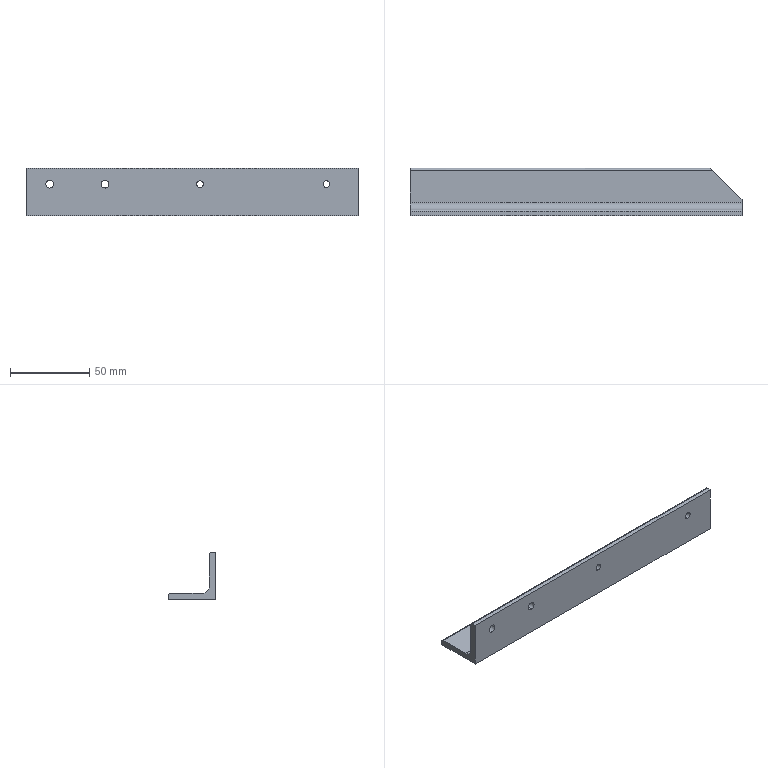Part | NX | features BREP 1 | 1 solid | 20 faces | box 210 x 30 x 30 mm | volume 46732 mm3 | cylinder 11 | plane 9 | commonest cylinder face diameters 4.2 x4 5 x4 2.667 x2 9 x1
STEP:
#1=CARTESIAN_POINT('',(15.,4.,22.5));
#2=VERTEX_POINT('',#1);
#3=CARTESIAN_POINT('',(15.,4.,17.5));
#4=VERTEX_POINT('',#3);
#5=CARTESIAN_POINT('',(15.,4.,20.));
#6=DIRECTION('',(0.,-1.,0.));
#7=DIRECTION('',(0.,0.,-1.));
#8=AXIS2_PLACEMENT_3D('',#5,#6,#7);
#9=CIRCLE('',#8,2.5);
#10=EDGE_CURVE('',#2,#4,#9,.T.);
#11=ORIENTED_EDGE('',*,*,#10,.F.);
#12=CARTESIAN_POINT('',(15.,0.,22.5));
#13=VERTEX_POINT('',#12);
#14=CARTESIAN_POINT('',(15.,0.,22.5));
#15=DIRECTION('',(0.,-1.,0.));
#16=VECTOR('',#15,1000.);
#17=LINE('',#14,#16);
#18=EDGE_CURVE('',#2,#13,#17,.T.);
#19=ORIENTED_EDGE('',*,*,#18,.T.);
#20=CARTESIAN_POINT('',(15.,0.,17.5));
#21=VERTEX_POINT('',#20);
#22=CARTESIAN_POINT('',(15.,0.,20.));
#23=DIRECTION('',(0.,-1.,0.));
#24=DIRECTION('',(0.,0.,-1.));
#25=AXIS2_PLACEMENT_3D('',#22,#23,#24);
#26=CIRCLE('',#25,2.5);
#27=EDGE_CURVE('',#13,#21,#26,.T.);
#28=ORIENTED_EDGE('',*,*,#27,.T.);
#29=CARTESIAN_POINT('',(15.,0.,17.5));
#30=DIRECTION('',(0.,-1.,0.));
#31=VECTOR('',#30,1000.);
#32=LINE('',#29,#31);
#33=EDGE_CURVE('',#4,#21,#32,.T.);
#34=ORIENTED_EDGE('',*,*,#33,.F.);
#35=EDGE_LOOP('',(#11,#19,#28,#34));
#36=FACE_BOUND('',#35,.T.);
#37=CARTESIAN_POINT('',(15.,0.,20.));
#38=DIRECTION('',(0.,-1.,0.));
#39=DIRECTION('',(0.,0.,-1.));
#40=AXIS2_PLACEMENT_3D('',#37,#38,#39);
#41=CYLINDRICAL_SURFACE('',#40,2.5);
#42=ADVANCED_FACE('',(#36),#41,.F.);
#43=CARTESIAN_POINT('',(50.,4.,22.5));
#44=VERTEX_POINT('',#43);
#45=CARTESIAN_POINT('',(50.,4.,17.5));
#46=VERTEX_POINT('',#45);
#47=CARTESIAN_POINT('',(50.,4.,20.));
#48=DIRECTION('',(0.,-1.,0.));
#49=DIRECTION('',(0.,0.,-1.));
#50=AXIS2_PLACEMENT_3D('',#47,#48,#49);
#51=CIRCLE('',#50,2.5);
#52=EDGE_CURVE('',#44,#46,#51,.T.);
#53=ORIENTED_EDGE('',*,*,#52,.F.);
#54=CARTESIAN_POINT('',(50.,0.,22.5));
#55=VERTEX_POINT('',#54);
#56=CARTESIAN_POINT('',(50.,0.,22.5));
#57=DIRECTION('',(0.,-1.,0.));
#58=VECTOR('',#57,1000.);
#59=LINE('',#56,#58);
#60=EDGE_CURVE('',#44,#55,#59,.T.);
#61=ORIENTED_EDGE('',*,*,#60,.T.);
#62=CARTESIAN_POINT('',(50.,0.,17.5));
#63=VERTEX_POINT('',#62);
#64=CARTESIAN_POINT('',(50.,0.,20.));
#65=DIRECTION('',(0.,-1.,0.));
#66=DIRECTION('',(0.,0.,-1.));
#67=AXIS2_PLACEMENT_3D('',#64,#65,#66);
#68=CIRCLE('',#67,2.5);
#69=EDGE_CURVE('',#55,#63,#68,.T.);
#70=ORIENTED_EDGE('',*,*,#69,.T.);
#71=CARTESIAN_POINT('',(50.,0.,17.5));
#72=DIRECTION('',(0.,-1.,0.));
#73=VECTOR('',#72,1000.);
#74=LINE('',#71,#73);
#75=EDGE_CURVE('',#46,#63,#74,.T.);
#76=ORIENTED_EDGE('',*,*,#75,.F.);
#77=EDGE_LOOP('',(#53,#61,#70,#76));
#78=FACE_BOUND('',#77,.T.);
#79=CARTESIAN_POINT('',(50.,0.,20.));
#80=DIRECTION('',(0.,-1.,0.));
#81=DIRECTION('',(0.,0.,-1.));
#82=AXIS2_PLACEMENT_3D('',#79,#80,#81);
#83=CYLINDRICAL_SURFACE('',#82,2.5);
#84=ADVANCED_FACE('',(#78),#83,.F.);
#85=CARTESIAN_POINT('',(190.,4.,22.1));
#86=VERTEX_POINT('',#85);
#87=CARTESIAN_POINT('',(190.,4.,17.9));
#88=VERTEX_POINT('',#87);
#89=CARTESIAN_POINT('',(190.,4.,20.));
#90=DIRECTION('',(0.,-1.,0.));
#91=DIRECTION('',(0.,0.,-1.));
#92=AXIS2_PLACEMENT_3D('',#89,#90,#91);
#93=CIRCLE('',#92,2.1);
#94=EDGE_CURVE('',#86,#88,#93,.T.);
#95=ORIENTED_EDGE('',*,*,#94,.F.);
#96=CARTESIAN_POINT('',(190.,0.,22.1));
#97=VERTEX_POINT('',#96);
#98=CARTESIAN_POINT('',(190.,0.,22.1));
#99=DIRECTION('',(0.,-1.,0.));
#100=VECTOR('',#99,1000.);
#101=LINE('',#98,#100);
#102=EDGE_CURVE('',#86,#97,#101,.T.);
#103=ORIENTED_EDGE('',*,*,#102,.T.);
#104=CARTESIAN_POINT('',(190.,0.,17.9));
#105=VERTEX_POINT('',#104);
#106=CARTESIAN_POINT('',(190.,0.,20.));
#107=DIRECTION('',(0.,-1.,0.));
#108=DIRECTION('',(0.,0.,-1.));
#109=AXIS2_PLACEMENT_3D('',#106,#107,#108);
#110=CIRCLE('',#109,2.1);
#111=EDGE_CURVE('',#97,#105,#110,.T.);
#112=ORIENTED_EDGE('',*,*,#111,.T.);
#113=CARTESIAN_POINT('',(190.,0.,17.9));
#114=DIRECTION('',(0.,-1.,0.));
#115=VECTOR('',#114,1000.);
#116=LINE('',#113,#115);
#117=EDGE_CURVE('',#88,#105,#116,.T.);
#118=ORIENTED_EDGE('',*,*,#117,.F.);
#119=EDGE_LOOP('',(#95,#103,#112,#118));
#120=FACE_BOUND('',#119,.T.);
#121=CARTESIAN_POINT('',(190.,0.,20.));
#122=DIRECTION('',(0.,-1.,0.));
#123=DIRECTION('',(0.,0.,-1.));
#124=AXIS2_PLACEMENT_3D('',#121,#122,#123);
#125=CYLINDRICAL_SURFACE('',#124,2.1);
#126=ADVANCED_FACE('',(#120),#125,.F.);
#127=CARTESIAN_POINT('',(110.,4.,22.1));
#128=VERTEX_POINT('',#127);
#129=CARTESIAN_POINT('',(110.,4.,17.9));
#130=VERTEX_POINT('',#129);
#131=CARTESIAN_POINT('',(110.,4.,20.));
#132=DIRECTION('',(0.,-1.,0.));
#133=DIRECTION('',(0.,0.,-1.));
#134=AXIS2_PLACEMENT_3D('',#131,#132,#133);
#135=CIRCLE('',#134,2.1);
#136=EDGE_CURVE('',#128,#130,#135,.T.);
#137=ORIENTED_EDGE('',*,*,#136,.F.);
#138=CARTESIAN_POINT('',(110.,0.,22.1));
#139=VERTEX_POINT('',#138);
#140=CARTESIAN_POINT('',(110.,0.,22.1));
#141=DIRECTION('',(0.,-1.,0.));
#142=VECTOR('',#141,1000.);
#143=LINE('',#140,#142);
#144=EDGE_CURVE('',#128,#139,#143,.T.);
#145=ORIENTED_EDGE('',*,*,#144,.T.);
#146=CARTESIAN_POINT('',(110.,0.,17.9));
#147=VERTEX_POINT('',#146);
#148=CARTESIAN_POINT('',(110.,0.,20.));
#149=DIRECTION('',(0.,-1.,0.));
#150=DIRECTION('',(0.,0.,-1.));
#151=AXIS2_PLACEMENT_3D('',#148,#149,#150);
#152=CIRCLE('',#151,2.1);
#153=EDGE_CURVE('',#139,#147,#152,.T.);
#154=ORIENTED_EDGE('',*,*,#153,.T.);
#155=CARTESIAN_POINT('',(110.,0.,17.9));
#156=DIRECTION('',(0.,-1.,0.));
#157=VECTOR('',#156,1000.);
#158=LINE('',#155,#157);
#159=EDGE_CURVE('',#130,#147,#158,.T.);
#160=ORIENTED_EDGE('',*,*,#159,.F.);
#161=EDGE_LOOP('',(#137,#145,#154,#160));
#162=FACE_BOUND('',#161,.T.);
#163=CARTESIAN_POINT('',(110.,0.,20.));
#164=DIRECTION('',(0.,-1.,0.));
#165=DIRECTION('',(0.,0.,-1.));
#166=AXIS2_PLACEMENT_3D('',#163,#164,#165);
#167=CYLINDRICAL_SURFACE('',#166,2.1);
#168=ADVANCED_FACE('',(#162),#167,.F.);
#169=CARTESIAN_POINT('',(0.,0.,30.));
#170=VERTEX_POINT('',#169);
#171=CARTESIAN_POINT('',(0.,0.,0.));
#172=VERTEX_POINT('',#171);
#173=CARTESIAN_POINT('',(0.,0.,0.));
#174=DIRECTION('',(0.,0.,-1.));
#175=VECTOR('',#174,1000.);
#176=LINE('',#173,#175);
#177=EDGE_CURVE('',#170,#172,#176,.T.);
#178=ORIENTED_EDGE('',*,*,#177,.T.);
#179=CARTESIAN_POINT('',(210.,0.,0.));
#180=VERTEX_POINT('',#179);
#181=CARTESIAN_POINT('',(210.,0.,0.));
#182=DIRECTION('',(-1.,0.,0.));
#183=VECTOR('',#182,1000.);
#184=LINE('',#181,#183);
#185=EDGE_CURVE('',#180,#172,#184,.T.);
#186=ORIENTED_EDGE('',*,*,#185,.F.);
#187=CARTESIAN_POINT('',(210.,0.,30.));
#188=VERTEX_POINT('',#187);
#189=CARTESIAN_POINT('',(210.,0.,0.));
#190=DIRECTION('',(0.,0.,-1.));
#191=VECTOR('',#190,1000.);
#192=LINE('',#189,#191);
#193=EDGE_CURVE('',#188,#180,#192,.T.);
#194=ORIENTED_EDGE('',*,*,#193,.F.);
#195=CARTESIAN_POINT('',(210.,0.,30.));
#196=DIRECTION('',(-1.,0.,0.));
#197=VECTOR('',#196,1000.);
#198=LINE('',#195,#197);
#199=EDGE_CURVE('',#188,#170,#198,.T.);
#200=ORIENTED_EDGE('',*,*,#199,.T.);
#201=EDGE_LOOP('',(#178,#186,#194,#200));
#202=FACE_BOUND('',#201,.T.);
#203=CARTESIAN_POINT('',(15.,0.,20.));
#204=DIRECTION('',(0.,-1.,0.));
#205=DIRECTION('',(0.,0.,-1.));
#206=AXIS2_PLACEMENT_3D('',#203,#204,#205);
#207=CIRCLE('',#206,2.5);
#208=EDGE_CURVE('',#21,#13,#207,.T.);
#209=ORIENTED_EDGE('',*,*,#208,.F.);
#210=ORIENTED_EDGE('',*,*,#27,.F.);
#211=EDGE_LOOP('',(#209,#210));
#212=FACE_BOUND('',#211,.T.);
#213=CARTESIAN_POINT('',(50.,0.,20.));
#214=DIRECTION('',(0.,-1.,0.));
#215=DIRECTION('',(0.,0.,-1.));
#216=AXIS2_PLACEMENT_3D('',#213,#214,#215);
#217=CIRCLE('',#216,2.5);
#218=EDGE_CURVE('',#63,#55,#217,.T.);
#219=ORIENTED_EDGE('',*,*,#218,.F.);
#220=ORIENTED_EDGE('',*,*,#69,.F.);
#221=EDGE_LOOP('',(#219,#220));
#222=FACE_BOUND('',#221,.T.);
#223=CARTESIAN_POINT('',(190.,0.,20.));
#224=DIRECTION('',(0.,-1.,0.));
#225=DIRECTION('',(0.,0.,-1.));
#226=AXIS2_PLACEMENT_3D('',#223,#224,#225);
#227=CIRCLE('',#226,2.1);
#228=EDGE_CURVE('',#105,#97,#227,.T.);
#229=ORIENTED_EDGE('',*,*,#228,.F.);
#230=ORIENTED_EDGE('',*,*,#111,.F.);
#231=EDGE_LOOP('',(#229,#230));
#232=FACE_BOUND('',#231,.T.);
#233=CARTESIAN_POINT('',(110.,0.,20.));
#234=DIRECTION('',(0.,-1.,0.));
#235=DIRECTION('',(0.,0.,-1.));
#236=AXIS2_PLACEMENT_3D('',#233,#234,#235);
#237=CIRCLE('',#236,2.1);
#238=EDGE_CURVE('',#147,#139,#237,.T.);
#239=ORIENTED_EDGE('',*,*,#238,.F.);
#240=ORIENTED_EDGE('',*,*,#153,.F.);
#241=EDGE_LOOP('',(#239,#240));
#242=FACE_BOUND('',#241,.T.);
#243=CARTESIAN_POINT('',(210.,0.,0.));
#244=DIRECTION('',(0.,1.,0.));
#245=DIRECTION('',(1.,0.,0.));
#246=AXIS2_PLACEMENT_3D('',#243,#244,#245);
#247=PLANE('',#246);
#248=ADVANCED_FACE('',(#202,#212,#222,#232,#242),#247,.F.);
#249=CARTESIAN_POINT('',(190.,30.,0.));
#250=VERTEX_POINT('',#249);
#251=CARTESIAN_POINT('',(0.,30.,0.));
#252=VERTEX_POINT('',#251);
#253=CARTESIAN_POINT('',(210.,30.,0.));
#254=DIRECTION('',(-1.,0.,0.));
#255=VECTOR('',#254,1000.);
#256=LINE('',#253,#255);
#257=EDGE_CURVE('',#250,#252,#256,.T.);
#258=ORIENTED_EDGE('',*,*,#257,.F.);
#259=CARTESIAN_POINT('',(210.,10.,0.));
#260=VERTEX_POINT('',#259);
#261=CARTESIAN_POINT('',(210.,10.,0.));
#262=DIRECTION('',(0.7071,-0.7071,0.));
#263=VECTOR('',#262,1000.);
#264=LINE('',#261,#263);
#265=EDGE_CURVE('',#250,#260,#264,.T.);
#266=ORIENTED_EDGE('',*,*,#265,.T.);
#267=CARTESIAN_POINT('',(210.,0.,0.));
#268=DIRECTION('',(0.,1.,0.));
#269=VECTOR('',#268,1000.);
#270=LINE('',#267,#269);
#271=EDGE_CURVE('',#180,#260,#270,.T.);
#272=ORIENTED_EDGE('',*,*,#271,.F.);
#273=ORIENTED_EDGE('',*,*,#185,.T.);
#274=CARTESIAN_POINT('',(0.,0.,0.));
#275=DIRECTION('',(0.,1.,0.));
#276=VECTOR('',#275,1000.);
#277=LINE('',#274,#276);
#278=EDGE_CURVE('',#172,#252,#277,.T.);
#279=ORIENTED_EDGE('',*,*,#278,.T.);
#280=EDGE_LOOP('',(#258,#266,#272,#273,#279));
#281=FACE_BOUND('',#280,.T.);
#282=CARTESIAN_POINT('',(210.,0.,0.));
#283=DIRECTION('',(0.,0.,1.));
#284=DIRECTION('',(1.,0.,0.));
#285=AXIS2_PLACEMENT_3D('',#282,#283,#284);
#286=PLANE('',#285);
#287=ADVANCED_FACE('',(#281),#286,.F.);
#288=CARTESIAN_POINT('',(190.,30.,2.667));
#289=VERTEX_POINT('',#288);
#290=CARTESIAN_POINT('',(0.,30.,2.667));
#291=VERTEX_POINT('',#290);
#292=CARTESIAN_POINT('',(210.,30.,2.667));
#293=DIRECTION('',(-1.,0.,0.));
#294=VECTOR('',#293,1000.);
#295=LINE('',#292,#294);
#296=EDGE_CURVE('',#289,#291,#295,.T.);
#297=ORIENTED_EDGE('',*,*,#296,.F.);
#298=CARTESIAN_POINT('',(190.,30.,0.));
#299=DIRECTION('',(0.,0.,-1.));
#300=VECTOR('',#299,1000.);
#301=LINE('',#298,#300);
#302=EDGE_CURVE('',#289,#250,#301,.T.);
#303=ORIENTED_EDGE('',*,*,#302,.T.);
#304=ORIENTED_EDGE('',*,*,#257,.T.);
#305=CARTESIAN_POINT('',(0.,30.,0.));
#306=DIRECTION('',(0.,0.,1.));
#307=VECTOR('',#306,1000.);
#308=LINE('',#305,#307);
#309=EDGE_CURVE('',#252,#291,#308,.T.);
#310=ORIENTED_EDGE('',*,*,#309,.T.);
#311=EDGE_LOOP('',(#297,#303,#304,#310));
#312=FACE_BOUND('',#311,.T.);
#313=CARTESIAN_POINT('',(210.,30.,0.));
#314=DIRECTION('',(0.,-1.,0.));
#315=DIRECTION('',(0.,0.,-1.));
#316=AXIS2_PLACEMENT_3D('',#313,#314,#315);
#317=PLANE('',#316);
#318=ADVANCED_FACE('',(#312),#317,.F.);
#319=CARTESIAN_POINT('',(191.333,28.667,4.));
#320=VERTEX_POINT('',#319);
#321=CARTESIAN_POINT('',(0.,28.667,4.));
#322=VERTEX_POINT('',#321);
#323=CARTESIAN_POINT('',(210.,28.667,4.));
#324=DIRECTION('',(-1.,0.,0.));
#325=VECTOR('',#324,1000.);
#326=LINE('',#323,#325);
#327=EDGE_CURVE('',#320,#322,#326,.T.);
#328=ORIENTED_EDGE('',*,*,#327,.F.);
#329=CARTESIAN_POINT('',(191.333,28.667,4.));
#330=CARTESIAN_POINT('',(190.552,29.448,4.));
#331=CARTESIAN_POINT('',(190.,30.,3.448));
#332=CARTESIAN_POINT('',(190.,30.,2.667));
#333=(BOUNDED_CURVE()B_SPLINE_CURVE(3,(#329,#330,#331,#332),.UNSPECIFIED.,.F.,.F.)B_SPLINE_CURVE_WITH_KNOTS((4,4),(4.712,6.283),.UNSPECIFIED.)CURVE()GEOMETRIC_REPRESENTATION_ITEM()RATIONAL_B_SPLINE_CURVE((1.,0.8047,0.8047,1.))REPRESENTATION_ITEM(''));
#334=EDGE_CURVE('',#320,#289,#333,.T.);
#335=ORIENTED_EDGE('',*,*,#334,.T.);
#336=ORIENTED_EDGE('',*,*,#296,.T.);
#337=CARTESIAN_POINT('',(0.,28.667,2.667));
#338=DIRECTION('',(1.,0.,0.));
#339=DIRECTION('',(0.,0.,-1.));
#340=AXIS2_PLACEMENT_3D('',#337,#338,#339);
#341=CIRCLE('',#340,1.333);
#342=EDGE_CURVE('',#291,#322,#341,.T.);
#343=ORIENTED_EDGE('',*,*,#342,.T.);
#344=EDGE_LOOP('',(#328,#335,#336,#343));
#345=FACE_BOUND('',#344,.T.);
#346=CARTESIAN_POINT('',(210.,28.667,2.667));
#347=DIRECTION('',(-1.,0.,0.));
#348=DIRECTION('',(0.,0.,1.));
#349=AXIS2_PLACEMENT_3D('',#346,#347,#348);
#350=CYLINDRICAL_SURFACE('',#349,1.333);
#351=ADVANCED_FACE('',(#345),#350,.T.);
#352=CARTESIAN_POINT('',(210.,10.,4.));
#353=VERTEX_POINT('',#352);
#354=CARTESIAN_POINT('',(210.,8.5,4.));
#355=VERTEX_POINT('',#354);
#356=CARTESIAN_POINT('',(210.,8.5,4.));
#357=DIRECTION('',(0.,-1.,0.));
#358=VECTOR('',#357,1000.);
#359=LINE('',#356,#358);
#360=EDGE_CURVE('',#353,#355,#359,.T.);
#361=ORIENTED_EDGE('',*,*,#360,.F.);
#362=CARTESIAN_POINT('',(210.,10.,4.));
#363=DIRECTION('',(-0.7071,0.7071,0.));
#364=VECTOR('',#363,1000.);
#365=LINE('',#362,#364);
#366=EDGE_CURVE('',#353,#320,#365,.T.);
#367=ORIENTED_EDGE('',*,*,#366,.T.);
#368=ORIENTED_EDGE('',*,*,#327,.T.);
#369=CARTESIAN_POINT('',(0.,8.5,4.));
#370=VERTEX_POINT('',#369);
#371=CARTESIAN_POINT('',(0.,8.5,4.));
#372=DIRECTION('',(0.,-1.,0.));
#373=VECTOR('',#372,1000.);
#374=LINE('',#371,#373);
#375=EDGE_CURVE('',#322,#370,#374,.T.);
#376=ORIENTED_EDGE('',*,*,#375,.T.);
#377=CARTESIAN_POINT('',(210.,8.5,4.));
#378=DIRECTION('',(-1.,0.,0.));
#379=VECTOR('',#378,1000.);
#380=LINE('',#377,#379);
#381=EDGE_CURVE('',#355,#370,#380,.T.);
#382=ORIENTED_EDGE('',*,*,#381,.F.);
#383=EDGE_LOOP('',(#361,#367,#368,#376,#382));
#384=FACE_BOUND('',#383,.T.);
#385=CARTESIAN_POINT('',(210.,8.5,4.));
#386=DIRECTION('',(0.,0.,-1.));
#387=DIRECTION('',(0.,-1.,0.));
#388=AXIS2_PLACEMENT_3D('',#385,#386,#387);
#389=PLANE('',#388);
#390=ADVANCED_FACE('',(#384),#389,.F.);
#391=CARTESIAN_POINT('',(0.,4.,8.5));
#392=VERTEX_POINT('',#391);
#393=CARTESIAN_POINT('',(0.,8.5,8.5));
#394=DIRECTION('',(-1.,0.,0.));
#395=DIRECTION('',(0.,0.,-1.));
#396=AXIS2_PLACEMENT_3D('',#393,#394,#395);
#397=CIRCLE('',#396,4.5);
#398=EDGE_CURVE('',#370,#392,#397,.T.);
#399=ORIENTED_EDGE('',*,*,#398,.T.);
#400=CARTESIAN_POINT('',(210.,4.,8.5));
#401=VERTEX_POINT('',#400);
#402=CARTESIAN_POINT('',(210.,4.,8.5));
#403=DIRECTION('',(-1.,0.,0.));
#404=VECTOR('',#403,1000.);
#405=LINE('',#402,#404);
#406=EDGE_CURVE('',#401,#392,#405,.T.);
#407=ORIENTED_EDGE('',*,*,#406,.F.);
#408=CARTESIAN_POINT('',(210.,8.5,8.5));
#409=DIRECTION('',(-1.,0.,0.));
#410=DIRECTION('',(0.,0.,-1.));
#411=AXIS2_PLACEMENT_3D('',#408,#409,#410);
#412=CIRCLE('',#411,4.5);
#413=EDGE_CURVE('',#355,#401,#412,.T.);
#414=ORIENTED_EDGE('',*,*,#413,.F.);
#415=ORIENTED_EDGE('',*,*,#381,.T.);
#416=EDGE_LOOP('',(#399,#407,#414,#415));
#417=FACE_BOUND('',#416,.T.);
#418=CARTESIAN_POINT('',(210.,8.5,8.5));
#419=DIRECTION('',(-1.,0.,0.));
#420=DIRECTION('',(0.,0.,1.));
#421=AXIS2_PLACEMENT_3D('',#418,#419,#420);
#422=CYLINDRICAL_SURFACE('',#421,4.5);
#423=ADVANCED_FACE('',(#417),#422,.F.);
#424=CARTESIAN_POINT('',(0.,4.,28.667));
#425=VERTEX_POINT('',#424);
#426=CARTESIAN_POINT('',(0.,4.,28.667));
#427=DIRECTION('',(0.,0.,1.));
#428=VECTOR('',#427,1000.);
#429=LINE('',#426,#428);
#430=EDGE_CURVE('',#392,#425,#429,.T.);
#431=ORIENTED_EDGE('',*,*,#430,.T.);
#432=CARTESIAN_POINT('',(210.,4.,28.667));
#433=VERTEX_POINT('',#432);
#434=CARTESIAN_POINT('',(210.,4.,28.667));
#435=DIRECTION('',(-1.,0.,0.));
#436=VECTOR('',#435,1000.);
#437=LINE('',#434,#436);
#438=EDGE_CURVE('',#433,#425,#437,.T.);
#439=ORIENTED_EDGE('',*,*,#438,.F.);
#440=CARTESIAN_POINT('',(210.,4.,28.667));
#441=DIRECTION('',(0.,0.,1.));
#442=VECTOR('',#441,1000.);
#443=LINE('',#440,#442);
#444=EDGE_CURVE('',#401,#433,#443,.T.);
#445=ORIENTED_EDGE('',*,*,#444,.F.);
#446=ORIENTED_EDGE('',*,*,#406,.T.);
#447=EDGE_LOOP('',(#431,#439,#445,#446));
#448=FACE_BOUND('',#447,.T.);
#449=CARTESIAN_POINT('',(15.,4.,20.));
#450=DIRECTION('',(0.,-1.,0.));
#451=DIRECTION('',(0.,0.,-1.));
#452=AXIS2_PLACEMENT_3D('',#449,#450,#451);
#453=CIRCLE('',#452,2.5);
#454=EDGE_CURVE('',#4,#2,#453,.T.);
#455=ORIENTED_EDGE('',*,*,#454,.T.);
#456=ORIENTED_EDGE('',*,*,#10,.T.);
#457=EDGE_LOOP('',(#455,#456));
#458=FACE_BOUND('',#457,.T.);
#459=CARTESIAN_POINT('',(50.,4.,20.));
#460=DIRECTION('',(0.,-1.,0.));
#461=DIRECTION('',(0.,0.,-1.));
#462=AXIS2_PLACEMENT_3D('',#459,#460,#461);
#463=CIRCLE('',#462,2.5);
#464=EDGE_CURVE('',#46,#44,#463,.T.);
#465=ORIENTED_EDGE('',*,*,#464,.T.);
#466=ORIENTED_EDGE('',*,*,#52,.T.);
#467=EDGE_LOOP('',(#465,#466));
#468=FACE_BOUND('',#467,.T.);
#469=CARTESIAN_POINT('',(190.,4.,20.));
#470=DIRECTION('',(0.,-1.,0.));
#471=DIRECTION('',(0.,0.,-1.));
#472=AXIS2_PLACEMENT_3D('',#469,#470,#471);
#473=CIRCLE('',#472,2.1);
#474=EDGE_CURVE('',#88,#86,#473,.T.);
#475=ORIENTED_EDGE('',*,*,#474,.T.);
#476=ORIENTED_EDGE('',*,*,#94,.T.);
#477=EDGE_LOOP('',(#475,#476));
#478=FACE_BOUND('',#477,.T.);
#479=CARTESIAN_POINT('',(110.,4.,20.));
#480=DIRECTION('',(0.,-1.,0.));
#481=DIRECTION('',(0.,0.,-1.));
#482=AXIS2_PLACEMENT_3D('',#479,#480,#481);
#483=CIRCLE('',#482,2.1);
#484=EDGE_CURVE('',#130,#128,#483,.T.);
#485=ORIENTED_EDGE('',*,*,#484,.T.);
#486=ORIENTED_EDGE('',*,*,#136,.T.);
#487=EDGE_LOOP('',(#485,#486));
#488=FACE_BOUND('',#487,.T.);
#489=CARTESIAN_POINT('',(210.,4.,28.667));
#490=DIRECTION('',(0.,-1.,0.));
#491=DIRECTION('',(0.,0.,-1.));
#492=AXIS2_PLACEMENT_3D('',#489,#490,#491);
#493=PLANE('',#492);
#494=ADVANCED_FACE('',(#448,#458,#468,#478,#488),#493,.F.);
#495=CARTESIAN_POINT('',(0.,2.667,30.));
#496=VERTEX_POINT('',#495);
#497=CARTESIAN_POINT('',(0.,2.667,28.667));
#498=DIRECTION('',(1.,0.,0.));
#499=DIRECTION('',(0.,0.,-1.));
#500=AXIS2_PLACEMENT_3D('',#497,#498,#499);
#501=CIRCLE('',#500,1.333);
#502=EDGE_CURVE('',#425,#496,#501,.T.);
#503=ORIENTED_EDGE('',*,*,#502,.T.);
#504=CARTESIAN_POINT('',(210.,2.667,30.));
#505=VERTEX_POINT('',#504);
#506=CARTESIAN_POINT('',(210.,2.667,30.));
#507=DIRECTION('',(-1.,0.,0.));
#508=VECTOR('',#507,1000.);
#509=LINE('',#506,#508);
#510=EDGE_CURVE('',#505,#496,#509,.T.);
#511=ORIENTED_EDGE('',*,*,#510,.F.);
#512=CARTESIAN_POINT('',(210.,2.667,28.667));
#513=DIRECTION('',(1.,0.,0.));
#514=DIRECTION('',(0.,0.,-1.));
#515=AXIS2_PLACEMENT_3D('',#512,#513,#514);
#516=CIRCLE('',#515,1.333);
#517=EDGE_CURVE('',#433,#505,#516,.T.);
#518=ORIENTED_EDGE('',*,*,#517,.F.);
#519=ORIENTED_EDGE('',*,*,#438,.T.);
#520=EDGE_LOOP('',(#503,#511,#518,#519));
#521=FACE_BOUND('',#520,.T.);
#522=CARTESIAN_POINT('',(210.,2.667,28.667));
#523=DIRECTION('',(-1.,0.,0.));
#524=DIRECTION('',(0.,0.,1.));
#525=AXIS2_PLACEMENT_3D('',#522,#523,#524);
#526=CYLINDRICAL_SURFACE('',#525,1.333);
#527=ADVANCED_FACE('',(#521),#526,.T.);
#528=CARTESIAN_POINT('',(0.,0.,30.));
#529=DIRECTION('',(0.,-1.,0.));
#530=VECTOR('',#529,1000.);
#531=LINE('',#528,#530);
#532=EDGE_CURVE('',#496,#170,#531,.T.);
#533=ORIENTED_EDGE('',*,*,#532,.T.);
#534=ORIENTED_EDGE('',*,*,#199,.F.);
#535=CARTESIAN_POINT('',(210.,0.,30.));
#536=DIRECTION('',(0.,-1.,0.));
#537=VECTOR('',#536,1000.);
#538=LINE('',#535,#537);
#539=EDGE_CURVE('',#505,#188,#538,.T.);
#540=ORIENTED_EDGE('',*,*,#539,.F.);
#541=ORIENTED_EDGE('',*,*,#510,.T.);
#542=EDGE_LOOP('',(#533,#534,#540,#541));
#543=FACE_BOUND('',#542,.T.);
#544=CARTESIAN_POINT('',(210.,0.,30.));
#545=DIRECTION('',(0.,0.,-1.));
#546=DIRECTION('',(0.,-1.,0.));
#547=AXIS2_PLACEMENT_3D('',#544,#545,#546);
#548=PLANE('',#547);
#549=ADVANCED_FACE('',(#543),#548,.F.);
#550=ORIENTED_EDGE('',*,*,#271,.T.);
#551=CARTESIAN_POINT('',(210.,10.,2.667));
#552=DIRECTION('',(0.,0.,1.));
#553=VECTOR('',#552,1000.);
#554=LINE('',#551,#553);
#555=EDGE_CURVE('',#260,#353,#554,.T.);
#556=ORIENTED_EDGE('',*,*,#555,.T.);
#557=ORIENTED_EDGE('',*,*,#360,.T.);
#558=ORIENTED_EDGE('',*,*,#413,.T.);
#559=ORIENTED_EDGE('',*,*,#444,.T.);
#560=ORIENTED_EDGE('',*,*,#517,.T.);
#561=ORIENTED_EDGE('',*,*,#539,.T.);
#562=ORIENTED_EDGE('',*,*,#193,.T.);
#563=EDGE_LOOP('',(#550,#556,#557,#558,#559,#560,#561,#562));
#564=FACE_BOUND('',#563,.T.);
#565=CARTESIAN_POINT('',(210.,2.667,28.667));
#566=DIRECTION('',(1.,0.,0.));
#567=DIRECTION('',(0.,1.,0.));
#568=AXIS2_PLACEMENT_3D('',#565,#566,#567);
#569=PLANE('',#568);
#570=ADVANCED_FACE('',(#564),#569,.T.);
#571=ORIENTED_EDGE('',*,*,#177,.F.);
#572=ORIENTED_EDGE('',*,*,#532,.F.);
#573=ORIENTED_EDGE('',*,*,#502,.F.);
#574=ORIENTED_EDGE('',*,*,#430,.F.);
#575=ORIENTED_EDGE('',*,*,#398,.F.);
#576=ORIENTED_EDGE('',*,*,#375,.F.);
#577=ORIENTED_EDGE('',*,*,#342,.F.);
#578=ORIENTED_EDGE('',*,*,#309,.F.);
#579=ORIENTED_EDGE('',*,*,#278,.F.);
#580=EDGE_LOOP('',(#571,#572,#573,#574,#575,#576,#577,#578,#579));
#581=FACE_BOUND('',#580,.T.);
#582=CARTESIAN_POINT('',(0.,2.667,28.667));
#583=DIRECTION('',(1.,0.,0.));
#584=DIRECTION('',(0.,1.,0.));
#585=AXIS2_PLACEMENT_3D('',#582,#583,#584);
#586=PLANE('',#585);
#587=ADVANCED_FACE('',(#581),#586,.F.);
#588=ORIENTED_EDGE('',*,*,#144,.F.);
#589=ORIENTED_EDGE('',*,*,#484,.F.);
#590=ORIENTED_EDGE('',*,*,#159,.T.);
#591=ORIENTED_EDGE('',*,*,#238,.T.);
#592=EDGE_LOOP('',(#588,#589,#590,#591));
#593=FACE_BOUND('',#592,.T.);
#594=CARTESIAN_POINT('',(110.,0.,20.));
#595=DIRECTION('',(0.,-1.,0.));
#596=DIRECTION('',(0.,0.,-1.));
#597=AXIS2_PLACEMENT_3D('',#594,#595,#596);
#598=CYLINDRICAL_SURFACE('',#597,2.1);
#599=ADVANCED_FACE('',(#593),#598,.F.);
#600=ORIENTED_EDGE('',*,*,#102,.F.);
#601=ORIENTED_EDGE('',*,*,#474,.F.);
#602=ORIENTED_EDGE('',*,*,#117,.T.);
#603=ORIENTED_EDGE('',*,*,#228,.T.);
#604=EDGE_LOOP('',(#600,#601,#602,#603));
#605=FACE_BOUND('',#604,.T.);
#606=CARTESIAN_POINT('',(190.,0.,20.));
#607=DIRECTION('',(0.,-1.,0.));
#608=DIRECTION('',(0.,0.,-1.));
#609=AXIS2_PLACEMENT_3D('',#606,#607,#608);
#610=CYLINDRICAL_SURFACE('',#609,2.1);
#611=ADVANCED_FACE('',(#605),#610,.F.);
#612=ORIENTED_EDGE('',*,*,#60,.F.);
#613=ORIENTED_EDGE('',*,*,#464,.F.);
#614=ORIENTED_EDGE('',*,*,#75,.T.);
#615=ORIENTED_EDGE('',*,*,#218,.T.);
#616=EDGE_LOOP('',(#612,#613,#614,#615));
#617=FACE_BOUND('',#616,.T.);
#618=CARTESIAN_POINT('',(50.,0.,20.));
#619=DIRECTION('',(0.,-1.,0.));
#620=DIRECTION('',(0.,0.,-1.));
#621=AXIS2_PLACEMENT_3D('',#618,#619,#620);
#622=CYLINDRICAL_SURFACE('',#621,2.5);
#623=ADVANCED_FACE('',(#617),#622,.F.);
#624=ORIENTED_EDGE('',*,*,#18,.F.);
#625=ORIENTED_EDGE('',*,*,#454,.F.);
#626=ORIENTED_EDGE('',*,*,#33,.T.);
#627=ORIENTED_EDGE('',*,*,#208,.T.);
#628=EDGE_LOOP('',(#624,#625,#626,#627));
#629=FACE_BOUND('',#628,.T.);
#630=CARTESIAN_POINT('',(15.,0.,20.));
#631=DIRECTION('',(0.,-1.,0.));
#632=DIRECTION('',(0.,0.,-1.));
#633=AXIS2_PLACEMENT_3D('',#630,#631,#632);
#634=CYLINDRICAL_SURFACE('',#633,2.5);
#635=ADVANCED_FACE('',(#629),#634,.F.);
#636=ORIENTED_EDGE('',*,*,#265,.F.);
#637=ORIENTED_EDGE('',*,*,#302,.F.);
#638=ORIENTED_EDGE('',*,*,#334,.F.);
#639=ORIENTED_EDGE('',*,*,#366,.F.);
#640=ORIENTED_EDGE('',*,*,#555,.F.);
#641=EDGE_LOOP('',(#636,#637,#638,#639,#640));
#642=FACE_BOUND('',#641,.T.);
#643=CARTESIAN_POINT('',(210.,10.,28.667));
#644=DIRECTION('',(0.7071,0.7071,0.));
#645=DIRECTION('',(0.,0.,-1.));
#646=AXIS2_PLACEMENT_3D('',#643,#644,#645);
#647=PLANE('',#646);
#648=ADVANCED_FACE('',(#642),#647,.T.);
#649=CLOSED_SHELL('',(#42,#84,#126,#168,#248,#287,#318,#351,#390,#423,#494,#527,#549,#570,#587,#599,#611,#623,#635,#648));
#650=MANIFOLD_SOLID_BREP('',#649);
#651=(LENGTH_UNIT()NAMED_UNIT(*)SI_UNIT(.MILLI.,.METRE.));
#652=UNCERTAINTY_MEASURE_WITH_UNIT(LENGTH_MEASURE(0.00001),#651,'','');
#653=(NAMED_UNIT(*)PLANE_ANGLE_UNIT()SI_UNIT($,.RADIAN.));
#654=(NAMED_UNIT(*)SI_UNIT($,.STERADIAN.)SOLID_ANGLE_UNIT());
#655=(GEOMETRIC_REPRESENTATION_CONTEXT(3)GLOBAL_UNCERTAINTY_ASSIGNED_CONTEXT((#652))GLOBAL_UNIT_ASSIGNED_CONTEXT((#651,#653,#654))REPRESENTATION_CONTEXT('',''));
#656=ADVANCED_BREP_SHAPE_REPRESENTATION('',(#650),#655);